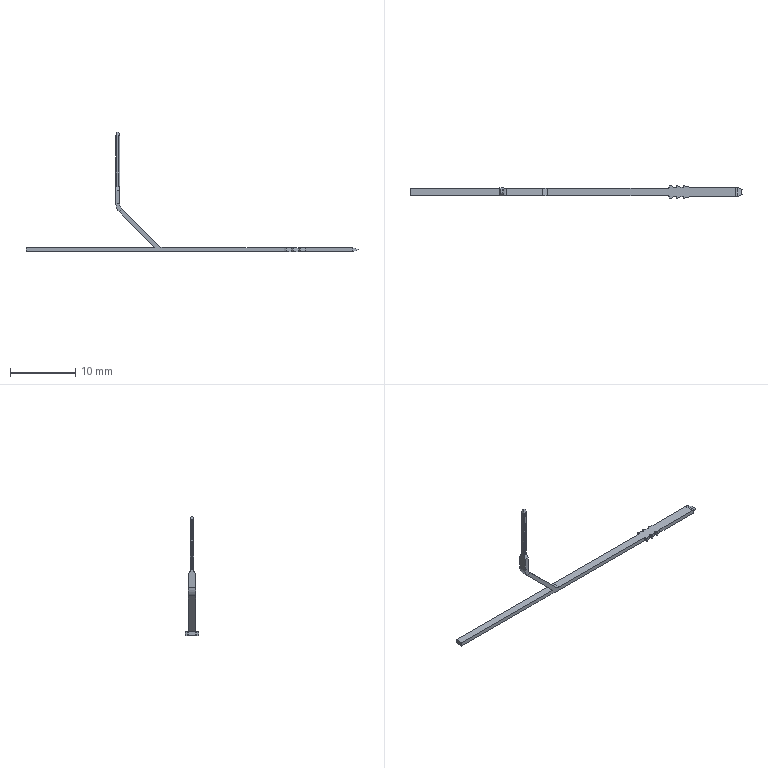Part | NX | features BREP 1 | 1 solid | 74 faces | box 51.003 x 2.1 x 18.3 mm | volume 49.874 mm3 | plane 42 | cylinder 32 | commonest cylinder face diameters 0.3 x12 0.2 x9 0.04 x4 0.025 x2 2 x2 2.4 x2